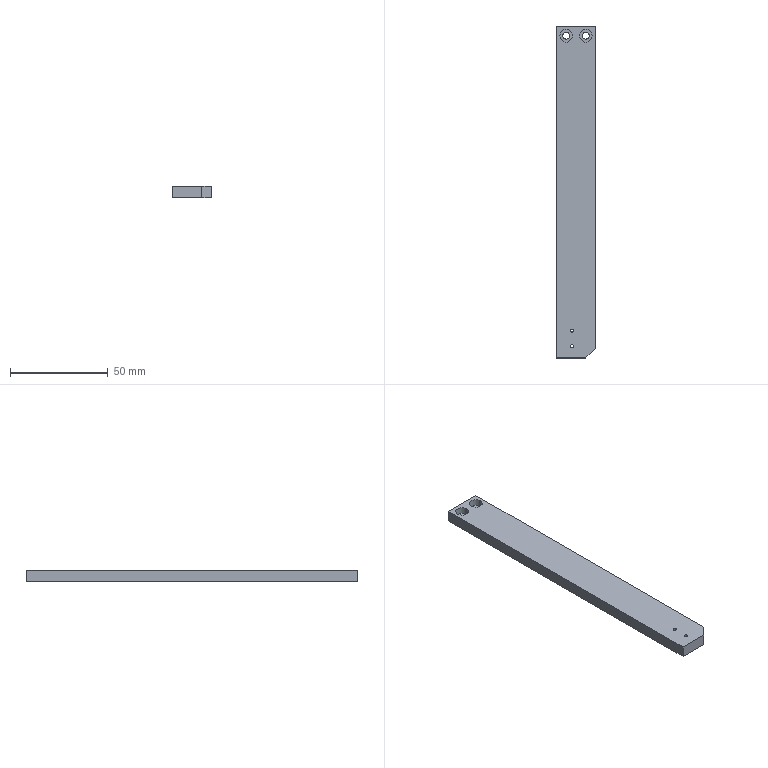Part | STEP file | 0232_210_Plate | 1 solid | 21 faces | box 20 x 170 x 6 mm | volume 20020 mm3 | cylinder 12 | plane 9 | commonest cylinder face diameters 1.6 x4 3.5 x4 6.5 x4